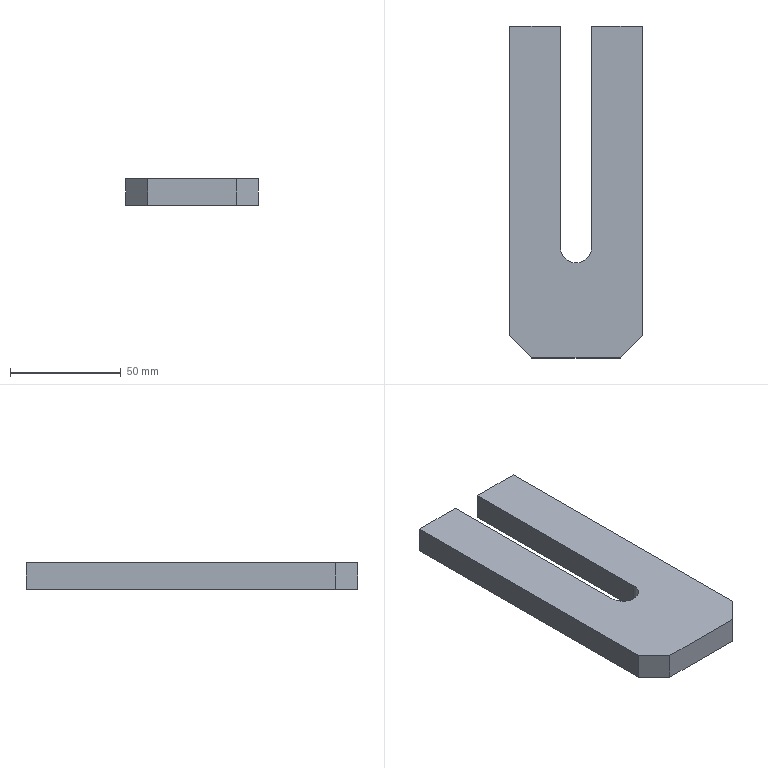Part | SolidWorks | features BaseBody 1 | 1 solid | 12 faces | box 60 x 150 x 12 mm | volume 89076 mm3 | plane 11 | cylinder 1 | commonest cylinder face diameters 14 x1
STEP:
#1=CARTESIAN_POINT('',(-30.,-65.,12.));
#2=VERTEX_POINT('',#1);
#3=CARTESIAN_POINT('',(-20.,-75.,12.));
#4=VERTEX_POINT('',#3);
#5=CARTESIAN_POINT('',(-30.,-65.,12.));
#6=DIRECTION('',(0.7071,-0.7071,0.));
#7=VECTOR('',#6,1000.);
#8=LINE('',#5,#7);
#9=EDGE_CURVE('',#2,#4,#8,.T.);
#10=ORIENTED_EDGE('',*,*,#9,.T.);
#11=CARTESIAN_POINT('',(20.,-75.,12.));
#12=VERTEX_POINT('',#11);
#13=CARTESIAN_POINT('',(0.,-75.,12.));
#14=DIRECTION('',(1.,0.,0.));
#15=VECTOR('',#14,1000.);
#16=LINE('',#13,#15);
#17=EDGE_CURVE('',#4,#12,#16,.T.);
#18=ORIENTED_EDGE('',*,*,#17,.T.);
#19=CARTESIAN_POINT('',(30.,-65.,12.));
#20=VERTEX_POINT('',#19);
#21=CARTESIAN_POINT('',(20.,-75.,12.));
#22=DIRECTION('',(0.7071,0.7071,0.));
#23=VECTOR('',#22,1000.);
#24=LINE('',#21,#23);
#25=EDGE_CURVE('',#12,#20,#24,.T.);
#26=ORIENTED_EDGE('',*,*,#25,.T.);
#27=CARTESIAN_POINT('',(30.,75.,12.));
#28=VERTEX_POINT('',#27);
#29=CARTESIAN_POINT('',(30.,5.274,12.));
#30=DIRECTION('',(0.,1.,0.));
#31=VECTOR('',#30,1000.);
#32=LINE('',#29,#31);
#33=EDGE_CURVE('',#20,#28,#32,.T.);
#34=ORIENTED_EDGE('',*,*,#33,.T.);
#35=CARTESIAN_POINT('',(7.,75.,12.));
#36=VERTEX_POINT('',#35);
#37=CARTESIAN_POINT('',(0.,75.,12.));
#38=DIRECTION('',(-1.,0.,0.));
#39=VECTOR('',#38,1000.);
#40=LINE('',#37,#39);
#41=EDGE_CURVE('',#28,#36,#40,.T.);
#42=ORIENTED_EDGE('',*,*,#41,.T.);
#43=CARTESIAN_POINT('',(7.,-25.,12.));
#44=VERTEX_POINT('',#43);
#45=CARTESIAN_POINT('',(7.,5.274,12.));
#46=DIRECTION('',(0.,-1.,0.));
#47=VECTOR('',#46,1000.);
#48=LINE('',#45,#47);
#49=EDGE_CURVE('',#36,#44,#48,.T.);
#50=ORIENTED_EDGE('',*,*,#49,.T.);
#51=CARTESIAN_POINT('',(-7.,-25.,12.));
#52=VERTEX_POINT('',#51);
#53=CARTESIAN_POINT('',(0.,-25.,12.));
#54=DIRECTION('',(0.,0.,-1.));
#55=DIRECTION('',(1.,0.,0.));
#56=AXIS2_PLACEMENT_3D('',#53,#54,#55);
#57=CIRCLE('',#56,7.);
#58=EDGE_CURVE('',#44,#52,#57,.T.);
#59=ORIENTED_EDGE('',*,*,#58,.T.);
#60=CARTESIAN_POINT('',(-7.,75.,12.));
#61=VERTEX_POINT('',#60);
#62=CARTESIAN_POINT('',(-7.,5.274,12.));
#63=DIRECTION('',(0.,1.,0.));
#64=VECTOR('',#63,1000.);
#65=LINE('',#62,#64);
#66=EDGE_CURVE('',#52,#61,#65,.T.);
#67=ORIENTED_EDGE('',*,*,#66,.T.);
#68=CARTESIAN_POINT('',(-30.,75.,12.));
#69=VERTEX_POINT('',#68);
#70=CARTESIAN_POINT('',(0.,75.,12.));
#71=DIRECTION('',(-1.,0.,0.));
#72=VECTOR('',#71,1000.);
#73=LINE('',#70,#72);
#74=EDGE_CURVE('',#61,#69,#73,.T.);
#75=ORIENTED_EDGE('',*,*,#74,.T.);
#76=CARTESIAN_POINT('',(-30.,5.274,12.));
#77=DIRECTION('',(0.,-1.,0.));
#78=VECTOR('',#77,1000.);
#79=LINE('',#76,#78);
#80=EDGE_CURVE('',#69,#2,#79,.T.);
#81=ORIENTED_EDGE('',*,*,#80,.T.);
#82=EDGE_LOOP('',(#10,#18,#26,#34,#42,#50,#59,#67,#75,#81));
#83=FACE_OUTER_BOUND('',#82,.T.);
#84=CARTESIAN_POINT('',(0.,5.274,12.));
#85=DIRECTION('',(0.,0.,1.));
#86=DIRECTION('',(1.,0.,0.));
#87=AXIS2_PLACEMENT_3D('',#84,#85,#86);
#88=PLANE('',#87);
#89=ADVANCED_FACE('',(#83),#88,.T.);
#90=CARTESIAN_POINT('',(-20.,-75.,0.));
#91=VERTEX_POINT('',#90);
#92=CARTESIAN_POINT('',(-20.,-75.,0.));
#93=DIRECTION('',(0.,0.,-1.));
#94=VECTOR('',#93,1000.);
#95=LINE('',#92,#94);
#96=EDGE_CURVE('',#4,#91,#95,.T.);
#97=ORIENTED_EDGE('',*,*,#96,.T.);
#98=CARTESIAN_POINT('',(20.,-75.,0.));
#99=VERTEX_POINT('',#98);
#100=CARTESIAN_POINT('',(30.,-75.,0.));
#101=DIRECTION('',(1.,0.,0.));
#102=VECTOR('',#101,1000.);
#103=LINE('',#100,#102);
#104=EDGE_CURVE('',#91,#99,#103,.T.);
#105=ORIENTED_EDGE('',*,*,#104,.T.);
#106=CARTESIAN_POINT('',(20.,-75.,0.));
#107=DIRECTION('',(0.,0.,1.));
#108=VECTOR('',#107,1000.);
#109=LINE('',#106,#108);
#110=EDGE_CURVE('',#99,#12,#109,.T.);
#111=ORIENTED_EDGE('',*,*,#110,.T.);
#112=ORIENTED_EDGE('',*,*,#17,.F.);
#113=EDGE_LOOP('',(#97,#105,#111,#112));
#114=FACE_OUTER_BOUND('',#113,.T.);
#115=CARTESIAN_POINT('',(30.,-75.,0.));
#116=DIRECTION('',(0.,-1.,0.));
#117=DIRECTION('',(1.,0.,0.));
#118=AXIS2_PLACEMENT_3D('',#115,#116,#117);
#119=PLANE('',#118);
#120=ADVANCED_FACE('',(#114),#119,.T.);
#121=CARTESIAN_POINT('',(-30.,-65.,0.));
#122=VERTEX_POINT('',#121);
#123=CARTESIAN_POINT('',(-25.,-70.,0.));
#124=DIRECTION('',(0.7071,-0.7071,0.));
#125=VECTOR('',#124,1000.);
#126=LINE('',#123,#125);
#127=EDGE_CURVE('',#122,#91,#126,.T.);
#128=ORIENTED_EDGE('',*,*,#127,.T.);
#129=ORIENTED_EDGE('',*,*,#96,.F.);
#130=ORIENTED_EDGE('',*,*,#9,.F.);
#131=CARTESIAN_POINT('',(-30.,-65.,0.));
#132=DIRECTION('',(0.,0.,-1.));
#133=VECTOR('',#132,1000.);
#134=LINE('',#131,#133);
#135=EDGE_CURVE('',#2,#122,#134,.T.);
#136=ORIENTED_EDGE('',*,*,#135,.T.);
#137=EDGE_LOOP('',(#128,#129,#130,#136));
#138=FACE_OUTER_BOUND('',#137,.T.);
#139=CARTESIAN_POINT('',(-25.,-70.,0.));
#140=DIRECTION('',(-0.7071,-0.7071,0.));
#141=DIRECTION('',(0.7071,-0.7071,0.));
#142=AXIS2_PLACEMENT_3D('',#139,#140,#141);
#143=PLANE('',#142);
#144=ADVANCED_FACE('',(#138),#143,.T.);
#145=CARTESIAN_POINT('',(-30.,75.,0.));
#146=VERTEX_POINT('',#145);
#147=CARTESIAN_POINT('',(-30.,75.,0.));
#148=DIRECTION('',(0.,0.,-1.));
#149=VECTOR('',#148,1000.);
#150=LINE('',#147,#149);
#151=EDGE_CURVE('',#69,#146,#150,.T.);
#152=ORIENTED_EDGE('',*,*,#151,.T.);
#153=CARTESIAN_POINT('',(-30.,-75.,0.));
#154=DIRECTION('',(0.,-1.,0.));
#155=VECTOR('',#154,1000.);
#156=LINE('',#153,#155);
#157=EDGE_CURVE('',#146,#122,#156,.T.);
#158=ORIENTED_EDGE('',*,*,#157,.T.);
#159=ORIENTED_EDGE('',*,*,#135,.F.);
#160=ORIENTED_EDGE('',*,*,#80,.F.);
#161=EDGE_LOOP('',(#152,#158,#159,#160));
#162=FACE_OUTER_BOUND('',#161,.T.);
#163=CARTESIAN_POINT('',(-30.,-75.,0.));
#164=DIRECTION('',(-1.,0.,0.));
#165=DIRECTION('',(0.,-1.,0.));
#166=AXIS2_PLACEMENT_3D('',#163,#164,#165);
#167=PLANE('',#166);
#168=ADVANCED_FACE('',(#162),#167,.T.);
#169=CARTESIAN_POINT('',(-7.,75.,0.));
#170=VERTEX_POINT('',#169);
#171=CARTESIAN_POINT('',(-30.,75.,0.));
#172=DIRECTION('',(-1.,0.,0.));
#173=VECTOR('',#172,1000.);
#174=LINE('',#171,#173);
#175=EDGE_CURVE('',#170,#146,#174,.T.);
#176=ORIENTED_EDGE('',*,*,#175,.T.);
#177=ORIENTED_EDGE('',*,*,#151,.F.);
#178=ORIENTED_EDGE('',*,*,#74,.F.);
#179=CARTESIAN_POINT('',(-7.,75.,0.));
#180=DIRECTION('',(0.,0.,-1.));
#181=VECTOR('',#180,1000.);
#182=LINE('',#179,#181);
#183=EDGE_CURVE('',#61,#170,#182,.T.);
#184=ORIENTED_EDGE('',*,*,#183,.T.);
#185=EDGE_LOOP('',(#176,#177,#178,#184));
#186=FACE_OUTER_BOUND('',#185,.T.);
#187=CARTESIAN_POINT('',(-30.,75.,0.));
#188=DIRECTION('',(0.,1.,0.));
#189=DIRECTION('',(0.,0.,1.));
#190=AXIS2_PLACEMENT_3D('',#187,#188,#189);
#191=PLANE('',#190);
#192=ADVANCED_FACE('',(#186),#191,.T.);
#193=CARTESIAN_POINT('',(-7.,-25.,0.));
#194=VERTEX_POINT('',#193);
#195=CARTESIAN_POINT('',(-7.,75.,0.));
#196=DIRECTION('',(0.,1.,0.));
#197=VECTOR('',#196,1000.);
#198=LINE('',#195,#197);
#199=EDGE_CURVE('',#194,#170,#198,.T.);
#200=ORIENTED_EDGE('',*,*,#199,.T.);
#201=ORIENTED_EDGE('',*,*,#183,.F.);
#202=ORIENTED_EDGE('',*,*,#66,.F.);
#203=CARTESIAN_POINT('',(-7.,-25.,0.));
#204=DIRECTION('',(0.,0.,-1.));
#205=VECTOR('',#204,1000.);
#206=LINE('',#203,#205);
#207=EDGE_CURVE('',#52,#194,#206,.T.);
#208=ORIENTED_EDGE('',*,*,#207,.T.);
#209=EDGE_LOOP('',(#200,#201,#202,#208));
#210=FACE_OUTER_BOUND('',#209,.T.);
#211=CARTESIAN_POINT('',(-7.,75.,0.));
#212=DIRECTION('',(1.,0.,0.));
#213=DIRECTION('',(0.,1.,0.));
#214=AXIS2_PLACEMENT_3D('',#211,#212,#213);
#215=PLANE('',#214);
#216=ADVANCED_FACE('',(#210),#215,.T.);
#217=CARTESIAN_POINT('',(7.,-25.,0.));
#218=VERTEX_POINT('',#217);
#219=CARTESIAN_POINT('',(7.,-25.,0.));
#220=DIRECTION('',(0.,0.,1.));
#221=VECTOR('',#220,1000.);
#222=LINE('',#219,#221);
#223=EDGE_CURVE('',#218,#44,#222,.T.);
#224=ORIENTED_EDGE('',*,*,#223,.F.);
#225=CARTESIAN_POINT('',(0.,-25.,0.));
#226=DIRECTION('',(0.,0.,1.));
#227=DIRECTION('',(1.,0.,0.));
#228=AXIS2_PLACEMENT_3D('',#225,#226,#227);
#229=CIRCLE('',#228,7.);
#230=EDGE_CURVE('',#194,#218,#229,.T.);
#231=ORIENTED_EDGE('',*,*,#230,.F.);
#232=ORIENTED_EDGE('',*,*,#207,.F.);
#233=ORIENTED_EDGE('',*,*,#58,.F.);
#234=EDGE_LOOP('',(#224,#231,#232,#233));
#235=FACE_OUTER_BOUND('',#234,.T.);
#236=CARTESIAN_POINT('',(0.,-25.,0.));
#237=DIRECTION('',(0.,0.,1.));
#238=DIRECTION('',(1.,0.,0.));
#239=AXIS2_PLACEMENT_3D('',#236,#237,#238);
#240=CYLINDRICAL_SURFACE('',#239,7.);
#241=ADVANCED_FACE('',(#235),#240,.F.);
#242=CARTESIAN_POINT('',(7.,75.,0.));
#243=VERTEX_POINT('',#242);
#244=CARTESIAN_POINT('',(7.,-25.,0.));
#245=DIRECTION('',(0.,-1.,0.));
#246=VECTOR('',#245,1000.);
#247=LINE('',#244,#246);
#248=EDGE_CURVE('',#243,#218,#247,.T.);
#249=ORIENTED_EDGE('',*,*,#248,.T.);
#250=ORIENTED_EDGE('',*,*,#223,.T.);
#251=ORIENTED_EDGE('',*,*,#49,.F.);
#252=CARTESIAN_POINT('',(7.,75.,0.));
#253=DIRECTION('',(0.,0.,-1.));
#254=VECTOR('',#253,1000.);
#255=LINE('',#252,#254);
#256=EDGE_CURVE('',#36,#243,#255,.T.);
#257=ORIENTED_EDGE('',*,*,#256,.T.);
#258=EDGE_LOOP('',(#249,#250,#251,#257));
#259=FACE_OUTER_BOUND('',#258,.T.);
#260=CARTESIAN_POINT('',(7.,-25.,0.));
#261=DIRECTION('',(-1.,0.,0.));
#262=DIRECTION('',(0.,-1.,0.));
#263=AXIS2_PLACEMENT_3D('',#260,#261,#262);
#264=PLANE('',#263);
#265=ADVANCED_FACE('',(#259),#264,.T.);
#266=CARTESIAN_POINT('',(30.,75.,0.));
#267=VERTEX_POINT('',#266);
#268=CARTESIAN_POINT('',(7.,75.,0.));
#269=DIRECTION('',(-1.,0.,0.));
#270=VECTOR('',#269,1000.);
#271=LINE('',#268,#270);
#272=EDGE_CURVE('',#267,#243,#271,.T.);
#273=ORIENTED_EDGE('',*,*,#272,.T.);
#274=ORIENTED_EDGE('',*,*,#256,.F.);
#275=ORIENTED_EDGE('',*,*,#41,.F.);
#276=CARTESIAN_POINT('',(30.,75.,0.));
#277=DIRECTION('',(0.,0.,-1.));
#278=VECTOR('',#277,1000.);
#279=LINE('',#276,#278);
#280=EDGE_CURVE('',#28,#267,#279,.T.);
#281=ORIENTED_EDGE('',*,*,#280,.T.);
#282=EDGE_LOOP('',(#273,#274,#275,#281));
#283=FACE_OUTER_BOUND('',#282,.T.);
#284=CARTESIAN_POINT('',(7.,75.,0.));
#285=DIRECTION('',(0.,1.,0.));
#286=DIRECTION('',(0.,0.,1.));
#287=AXIS2_PLACEMENT_3D('',#284,#285,#286);
#288=PLANE('',#287);
#289=ADVANCED_FACE('',(#283),#288,.T.);
#290=ORIENTED_EDGE('',*,*,#280,.F.);
#291=ORIENTED_EDGE('',*,*,#33,.F.);
#292=CARTESIAN_POINT('',(30.,-65.,0.));
#293=VERTEX_POINT('',#292);
#294=CARTESIAN_POINT('',(30.,-65.,0.));
#295=DIRECTION('',(0.,0.,-1.));
#296=VECTOR('',#295,1000.);
#297=LINE('',#294,#296);
#298=EDGE_CURVE('',#20,#293,#297,.T.);
#299=ORIENTED_EDGE('',*,*,#298,.T.);
#300=CARTESIAN_POINT('',(30.,75.,0.));
#301=DIRECTION('',(0.,1.,0.));
#302=VECTOR('',#301,1000.);
#303=LINE('',#300,#302);
#304=EDGE_CURVE('',#293,#267,#303,.T.);
#305=ORIENTED_EDGE('',*,*,#304,.T.);
#306=EDGE_LOOP('',(#290,#291,#299,#305));
#307=FACE_OUTER_BOUND('',#306,.T.);
#308=CARTESIAN_POINT('',(30.,75.,0.));
#309=DIRECTION('',(1.,0.,0.));
#310=DIRECTION('',(0.,1.,0.));
#311=AXIS2_PLACEMENT_3D('',#308,#309,#310);
#312=PLANE('',#311);
#313=ADVANCED_FACE('',(#307),#312,.T.);
#314=CARTESIAN_POINT('',(25.,-70.,0.));
#315=DIRECTION('',(0.7071,0.7071,0.));
#316=VECTOR('',#315,1000.);
#317=LINE('',#314,#316);
#318=EDGE_CURVE('',#99,#293,#317,.T.);
#319=ORIENTED_EDGE('',*,*,#318,.T.);
#320=ORIENTED_EDGE('',*,*,#298,.F.);
#321=ORIENTED_EDGE('',*,*,#25,.F.);
#322=ORIENTED_EDGE('',*,*,#110,.F.);
#323=EDGE_LOOP('',(#319,#320,#321,#322));
#324=FACE_OUTER_BOUND('',#323,.T.);
#325=CARTESIAN_POINT('',(25.,-70.,0.));
#326=DIRECTION('',(0.7071,-0.7071,0.));
#327=DIRECTION('',(0.7071,0.7071,0.));
#328=AXIS2_PLACEMENT_3D('',#325,#326,#327);
#329=PLANE('',#328);
#330=ADVANCED_FACE('',(#324),#329,.T.);
#331=ORIENTED_EDGE('',*,*,#104,.F.);
#332=ORIENTED_EDGE('',*,*,#127,.F.);
#333=ORIENTED_EDGE('',*,*,#157,.F.);
#334=ORIENTED_EDGE('',*,*,#175,.F.);
#335=ORIENTED_EDGE('',*,*,#199,.F.);
#336=ORIENTED_EDGE('',*,*,#230,.T.);
#337=ORIENTED_EDGE('',*,*,#248,.F.);
#338=ORIENTED_EDGE('',*,*,#272,.F.);
#339=ORIENTED_EDGE('',*,*,#304,.F.);
#340=ORIENTED_EDGE('',*,*,#318,.F.);
#341=EDGE_LOOP('',(#331,#332,#333,#334,#335,#336,#337,#338,#339,#340));
#342=FACE_OUTER_BOUND('',#341,.T.);
#343=CARTESIAN_POINT('',(0.,5.274,0.));
#344=DIRECTION('',(0.,0.,1.));
#345=DIRECTION('',(1.,0.,0.));
#346=AXIS2_PLACEMENT_3D('',#343,#344,#345);
#347=PLANE('',#346);
#348=ADVANCED_FACE('',(#342),#347,.F.);
#349=CLOSED_SHELL('',(#89,#120,#144,#168,#192,#216,#241,#265,#289,#313,#330,#348));
#350=MANIFOLD_SOLID_BREP('',#349);
#351=CARTESIAN_POINT('',(0.,0.,0.));
#352=DIRECTION('',(0.,0.,1.));
#353=DIRECTION('',(1.,0.,0.));
#354=AXIS2_PLACEMENT_3D('',#351,#352,#353);
#355=(LENGTH_UNIT()NAMED_UNIT(*)SI_UNIT(.MILLI.,.METRE.));
#356=UNCERTAINTY_MEASURE_WITH_UNIT(LENGTH_MEASURE(0.00001),#355,'','');
#357=(NAMED_UNIT(*)PLANE_ANGLE_UNIT()SI_UNIT($,.RADIAN.));
#358=(NAMED_UNIT(*)SI_UNIT($,.STERADIAN.)SOLID_ANGLE_UNIT());
#359=(GEOMETRIC_REPRESENTATION_CONTEXT(3)GLOBAL_UNCERTAINTY_ASSIGNED_CONTEXT((#356))GLOBAL_UNIT_ASSIGNED_CONTEXT((#355,#357,#358))REPRESENTATION_CONTEXT('',''));
#360=ADVANCED_BREP_SHAPE_REPRESENTATION('',(#350,#354),#359);